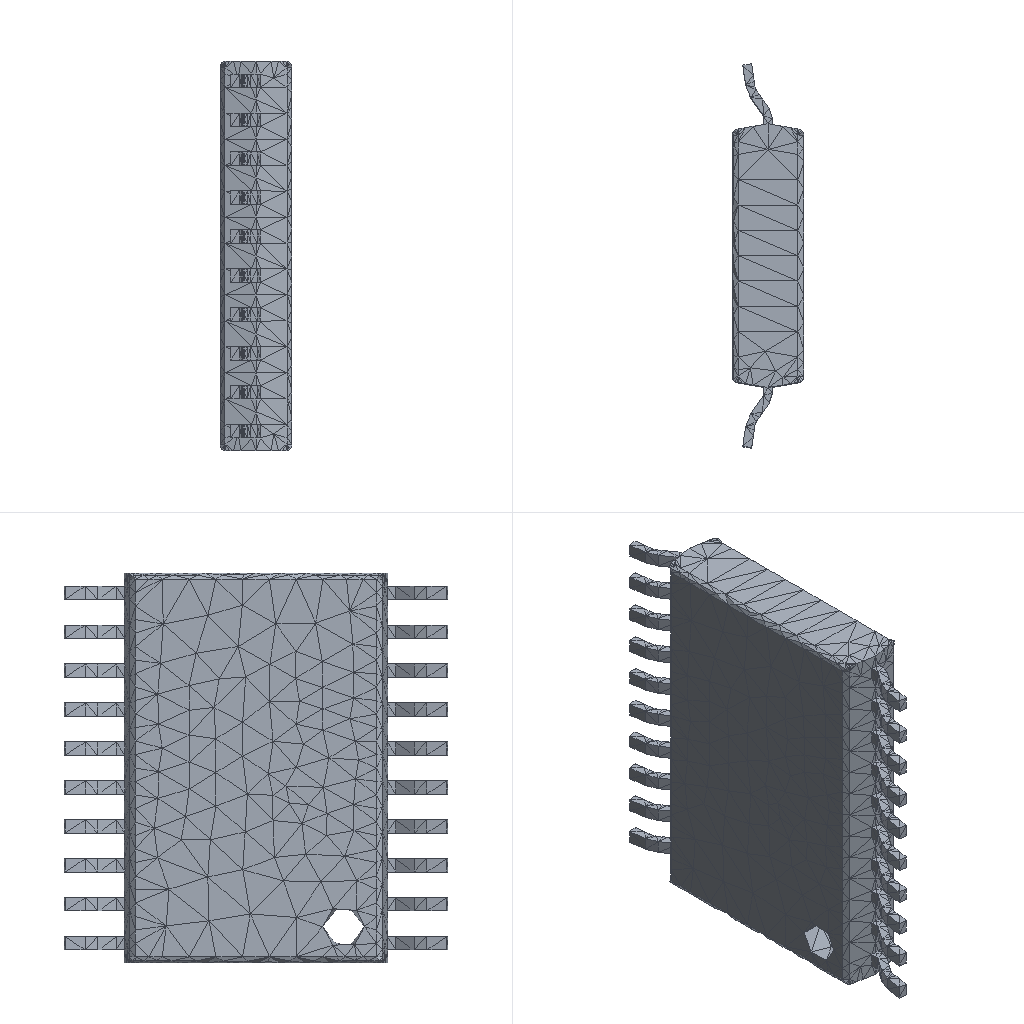Simulation study | ansys workbench
Set-up summary:
category,name,step,type,value,unit,region
solver,ansys_workbench
units,mm-N-s-tonne (MPa),,stated,"/units,MPA"
analysis,LS1,,static
load_step,LS1,LS1,static,nsubst=1; time=1
mesh,nodes,,,8744
mesh,elements,,,4480
element_type,SOLID187,,,4340
element_type,SURF154,,,140
material,Structural Steel,,E,200000,tonne s^-2 mm^-1
material,Structural Steel,,nu,0.3
material,Structural Steel,,density,7.85e-09,tonne mm^-3
material,Structural Steel,,conductivity,60.5,tonne mm s^-3 C^-1
material,Structural Steel,,specific_heat,4.34e+08,mm^2 s^-2 C^-1
material,Structural Steel,,cte,1.2e-05,C^-1
material,Structural Steel,,permeability,10000
material,Structural Steel,,resistivity,0.00017,ohm mm
load,Define Force Using Surface Effect Elements,LS1,surface-effect pres face 1,-5.813,,SURF154 #2
bc,Fixed Supports,model,fixed,[dofs=ALL],,_FIXEDSU
named_set,_FIXEDSU,,node,588
Ansys APDL input file, long lists of numbers shortened:
/batch
/config,noeldb,1     ! force off writing results to database
*get,_wallstrt,active,,time,wall
! ANSYS input file written by Workbench version 2024 R2
! File used for geometry attach:
/title,wbnew--____ (A5)
! ****** Begin Custom Load Command Snippet ******
/COM, ACT Extensions:
/COM,     LSDYNA, 2024.2
/COM,/COM,     ANSYSMotion, 2024.2
/COM,
! ****** End   Custom Load Command Snippet ******
*DIM,_wb_ProjectScratch_dir,string,248
_wb_ProjectScratch_dir(1) = ''
*DIM,_wb_SolverFiles_dir,string,248
_wb_SolverFiles_dir(1) = ''
*DIM,_wb_userfiles_dir,string,248
_wb_userfiles_dir(1) = ''
/com,--- Data in consistent NMM units. See Solving Units in the help system for more information.
/units,MPA
/nopr
/wb,file,start              !  signify a WB generated input file
/prep7
! Turn off shape checking because checks already performed inside WB mesher.
! See help system for more information.
SHPP,OFF,,NOWARN
/nolist
etcon,set             ! allow ANSYS to choose best KEYOP's for 180x elements, resets any applicable keyopt to MAPDL defaults
/com,*********** Nodes for the whole assembly ***********
nblock,3,,9618
(1i9,3e20.9e3)
        1     6.000000000E-01    -1.110293848E+00    -2.650000000E+00
! (8743 more lines like these left out)
-1
/wb,elem,start            !  set before creation of elements
/com,*********** Elements for Body 1 '__2-FreeParts|__-__2' ***********
et,1,187
eblock,19,solid,,4340
(19i9)
        1        1        1        1        0        0        0        0       10        0        1       69     1555      732     1437     2081     5826     2078     2079
! (8679 more lines like these left out)
-1
/wb,elem,end               !  done creating elements
/com,*********** Send User Defined Coordinate System(s) ***********
csys,0
toffst,273.15,      ! Temperature offset from absolute zero
/com,*********** Set Reference Temperature ***********
tref,22.
/wb,mat,start              !  starting to send materials
/com,*********** Send Materials ***********
Temperature = 'TEMP' ! Temperature
MP,DENS,1,7.85e-09,	! tonne mm^-3
MP,ALPX,1,1.2e-05,	! C^-1
MP,C,1,434000000,	! mm^2 s^-2 C^-1
MP,KXX,1,60.5,	! tonne mm s^-3 C^-1
MP,RSVX,1,0.00017,	! ohm mm
MP,EX,1,200000,	! tonne s^-2 mm^-1
MP,NUXY,1,0.3,
MP,MURX,1,10000,
/wb,mat,end                !  done sending materials
!************************* Model Summary ********************
!芯片2-FreeParts|切除-拉伸2,	结构钢,	matid,	1
!************************* End Model Summary ********************
! get the diagonal of the bounding box. Needed later for other things
*get,_xmin,node,,mnloc,x
*get,_ymin,node,,mnloc,y
*get,_zmin,node,,mnloc,z
*get,_xmax,node,,mxloc,x
*get,_ymax,node,,mxloc,y
*get,_zmax,node,,mxloc,z
_ASMDIAG=(_xmax-_xmin)*(_xmax-_xmin)+(_ymax-_ymin)*(_ymax-_ymin)+(_zmax-_zmin)*(_zmax-_zmin)
_ASMDIAG=SQRT(_ASMDIAG)
/wb,contact,start          !  starting to send contact
/wb,contact,end            !  done creating contacts
/golist
/wb,load,start             !  starting to send loads
/com,*********** Fixed Supports ***********
CMBLOCK,_FIXEDSU,NODE,      588
(8i10)
         1         2         3         4        95        96        97        98
! (73 more lines like these left out)
cmsel,s,_FIXEDSU
d,all,all
nsel,all
/com,*********** Define Force Using Surface Effect Elements ***********
local,12,0,0.,0.,0.,0.,0.,0.
csys,0
et,2,154
mat,2
eblock,10,,,140
(15i9)
     6913        2        2        2       12      599      593      985      985     5195     5197      985     5225
! (139 more lines like these left out)
-1
esel,s,type,,2
keyop,2,2,1         ! Apply load in local coordinate system
keyop,2,7,1         ! Use original area so load is constant in large deformation
esel,all
/gst,on,on
fini
*get,_numnode,node,0,count
*get,_numelem,elem,0,count
*get, _MAXELEMNUM, elem, 0, NUM, MAX
*get, _MAXNODENUM, node, 0, NUM, MAX
*get, _MAXELEMTYPE, etyp, 0, NUM, MAX
*get, _MAXREALCONST, rcon, 0, NUM, MAX
/go
/wb,load,end               !  done creating loads
/com,--- Number of total nodes = %_numnode%
/com,--- Number of contact elements = 140
/com,--- Number of spring elements = 0
/com,--- Number of bearing elements = 0
/com,--- Number of solid elements = 4340
/com,--- Number of condensed parts = 0
/com,--- Number of total elements = %_numelem%
*get,_wallbsol,active,,time,wall
/com,****************************************************************************
/com,*************************    SOLUTION       ********************************
/com,****************************************************************************
/solu
antype,0                   ! static analysis
_thickRatio=  1     ! Ratio of thick parts in the model
eqsl,pcg,1e-8,,,,,,1
cntr,print,1               ! print out contact info and also make no initial contact an error
cncheck,dmp		!	Enable program controlled contact splitting for distributed memory parallel run
dmpoption,emat,no             ! Don't combine emat file for DANSYS
dmpoption,esav,no             ! Don't combine esav file for DANSYS
nldiag,cont,iter           ! print out contact info each equilibrium iteration
rescontrol,,none                 ! Do not keep any restart files
/com,****************************************************
/com,******************* SOLVE FOR LS 1 OF 1 ****************
esel,s,type,,2
nsle
sfe,all,1,pres,1,-5.813
sfe,all,2,pres,1,0.
sfe,all,3,pres,1,0.
nsel,all
esel,all
/nopr
/gopr
nsub,1,1,1
time,1.
outres,erase
outres,all,none
outres,nsol,all,
outres,rsol,all
outres,eangl,all
outres,etmp,all
outres,veng,all
outres,strs,all,
outres,epel,all,
outres,eppl,all,
outres,cont,all,
! *********** WB SOLVE COMMAND ***********
! check interactive state
*get,ANSINTER_,active,,int
*if,ANSINTER_,ne,0,then
/eof
*endif
solve
/com *************** Write FE CONNECTORS *********
CEWRITE,file,ce,,INTE
/com,****************************************************
/com,*************** FINISHED SOLVE FOR LS 1 *************
*get,_wallasol,active,,time,wall
/nopr
*get,_numnode,node,0,count
*get,_numelem,elem,0,count
*get, _MAXELEMNUM, elem, 0, NUM, MAX
*get, _MAXNODENUM, node, 0, NUM, MAX,,,INTERNAL
*get, _MAXELEMTYPE, etyp, 0, NUM, MAX
*get, _MAXREALCONST, rcon, 0, NUM, MAX
*get,_NSOLTHREADS,active,0,ntfs
*get,_NSOLPROCESSES,active,0,npfs
/gopr
*get,_PCGITER,active,,solu,cgiter
/post1
xmlo,ENCODING,ISO-8859-1
xmlo,parm
/xml,parm,xml
fini
/gopr
*get,_walldone,active,,time,wall
_preptime=(_wallbsol-_wallstrt)*3600
_solvtime=(_wallasol-_wallbsol)*3600
_posttime=(_walldone-_wallasol)*3600
_totaltim=(_walldone-_wallstrt)*3600
*get,_dlbratio,active,0,solu,dlbr
*get,_combtime,active,0,solu,comb
*get,_ssmode,active,0,solu,ssmm
*get,_ndofs,active,0,solu,ndof
*get,_sol_end_time,active,0,set,time
*if,_sol_end_time,eq,1.,then
/fclean				!clean distributed files
*endif
/com,--- Total number of nodes = %_numnode%
/com,--- Total number of elements = %_numelem%
/com,--- Element load balance ratio = %_dlbratio%
/com,--- Time to combine distributed files = %_combtime%
/com,--- Sparse memory mode = %_ssmode%
/com,--- Number of DOF = %_ndofs%
/wb,file,end               ! done with WB generated input
Results summary:
result,analyses[0].index,,,1
result,analyses[0].system,,,SYS
result,analyses[0].deck,,,deck.dat
result,analyses[0].solve_status,,,completed
result,analyses[0].analysis_type,,,static
result,analyses[0].physics,,,mechanical
result,analyses[0].unit_system,,,"NMM: mm, ton, N, s, mV, mA, degC"
result,analyses[0].n_sets,,,1
result,analyses[0].load_steps[0].set,set=1,,1
result,analyses[0].load_steps[0].time_or_freq,set=1,,1
result,analyses[0].load_steps[0].max_displacement_magnitude,set=1,,0.01278
result,analyses[0].load_steps[0].max_von_mises_nodal,set=1,,468.652
result,analyses[0].load_steps[0].reaction_force_sum_xyz[1],set=1,,10
result,analyses[0].load_steps[0].reaction_force_sum_xyz[2],set=1,,-5.25245e-08
result,analyses[0].load_steps[0].reaction_force_sum_xyz[3],set=1,,5.34657e-08